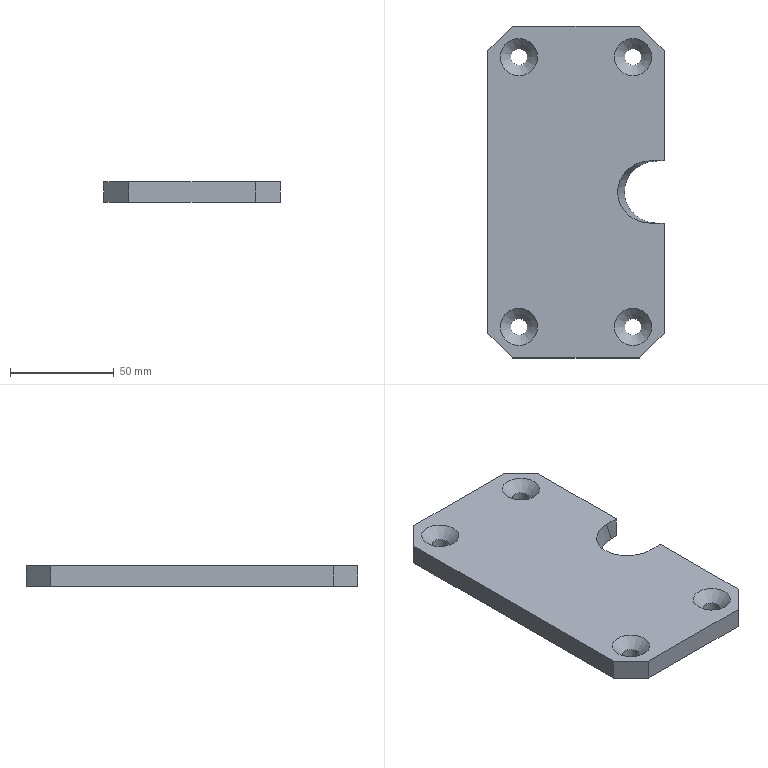Part | STEP file | solid 40 | 1 solid | 22 faces | box 85 x 160 x 10 mm | volume 124096 mm3 | plane 13 | cylinder 5 | cone 4 | commonest cylinder face diameters 8 x4 30 x1